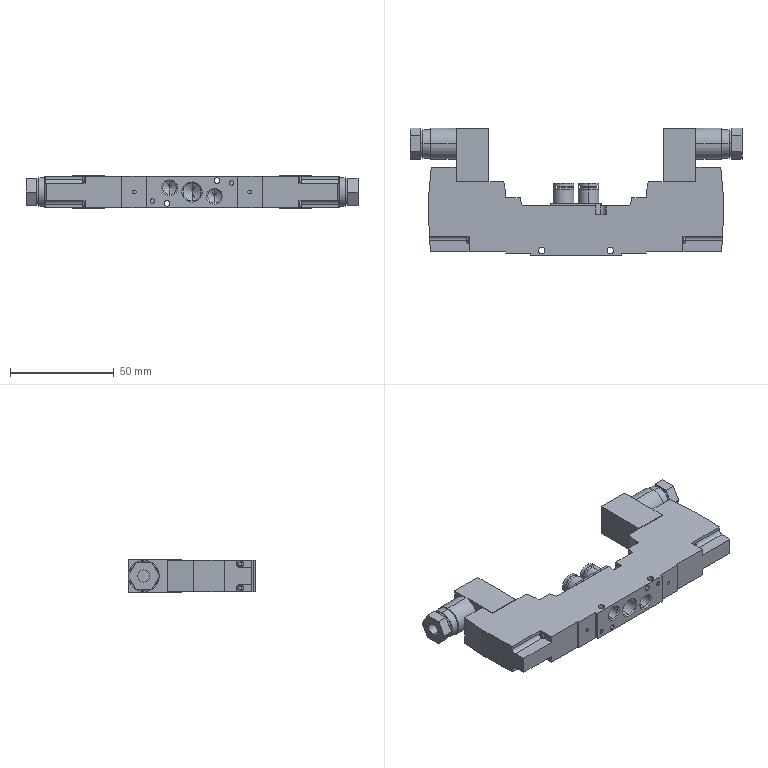Part | STEP file | VQZ2220-5YZ1-C6_V2_HI | 1 solid | 207 faces | box 159.8 x 61.406 x 15.8 mm | volume 81449 mm3 | plane 110 | cylinder 77 | cone 12 | torus 8 | commonest cylinder face diameters 3 x8 9.9 x8 1.8 x4 2.2 x4 2.7 x4 3.2 x4